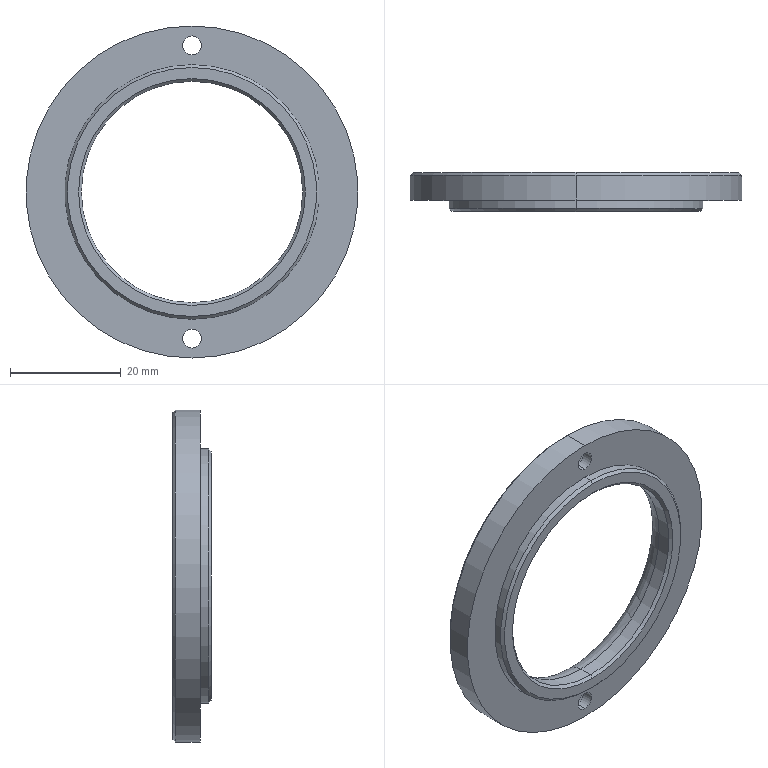Part | SolidWorks | features Chamfer 1, Extrusion 1, Fillet 1, HoleWzd 1, ICE 1 | 1 solid | 28 faces | box 60 x 7 x 60 mm | volume 7951 mm3 | cylinder 14 | cone 6 | plane 6 | torus 2 | commonest cylinder face diameters 3.4 x4 6 x4 40 x2 46 x2 60 x2
STEP:
#1=CARTESIAN_POINT('',(0.,0.5,23.5));
#2=VERTEX_POINT('',#1);
#3=CARTESIAN_POINT('',(0.,0.5,29.5));
#4=VERTEX_POINT('',#3);
#5=CARTESIAN_POINT('',(0.,0.5,26.5));
#6=DIRECTION('',(0.,1.,0.));
#7=DIRECTION('',(0.,0.,1.));
#8=AXIS2_PLACEMENT_3D('',#5,#6,#7);
#9=CIRCLE('',#8,3.);
#10=EDGE_CURVE('',#2,#4,#9,.T.);
#11=ORIENTED_EDGE('',*,*,#10,.F.);
#12=CARTESIAN_POINT('',(0.,3.469,23.5));
#13=VERTEX_POINT('',#12);
#14=CARTESIAN_POINT('',(0.,3.5,23.5));
#15=DIRECTION('',(0.,1.,0.));
#16=VECTOR('',#15,1000.);
#17=LINE('',#14,#16);
#18=EDGE_CURVE('',#2,#13,#17,.T.);
#19=ORIENTED_EDGE('',*,*,#18,.T.);
#20=CARTESIAN_POINT('',(-1.577,3.5,23.948));
#21=VERTEX_POINT('',#20);
#22=CARTESIAN_POINT('',(0.,3.469,23.5));
#23=CARTESIAN_POINT('',(-0.1379,3.469,23.5));
#24=CARTESIAN_POINT('',(-0.2777,3.47,23.51));
#25=CARTESIAN_POINT('',(-0.5518,3.475,23.548));
#26=CARTESIAN_POINT('',(-0.6865,3.479,23.576));
#27=CARTESIAN_POINT('',(-1.083,3.491,23.689));
#28=CARTESIAN_POINT('',(-1.341,3.5,23.802));
#29=CARTESIAN_POINT('',(-1.577,3.5,23.948));
#30=B_SPLINE_CURVE_WITH_KNOTS('',3,(#22,#23,#24,#25,#26,#27,#28,#29),.UNSPECIFIED.,.F.,.F.,(4,2,2,4),(0.00175,0.002163,0.002575,0.0034),.UNSPECIFIED.);
#31=EDGE_CURVE('',#13,#21,#30,.T.);
#32=ORIENTED_EDGE('',*,*,#31,.T.);
#33=CARTESIAN_POINT('',(0.,3.5,29.5));
#34=VERTEX_POINT('',#33);
#35=CARTESIAN_POINT('',(0.,3.5,26.5));
#36=DIRECTION('',(0.,1.,0.));
#37=DIRECTION('',(0.,0.,1.));
#38=AXIS2_PLACEMENT_3D('',#35,#36,#37);
#39=CIRCLE('',#38,3.);
#40=EDGE_CURVE('',#21,#34,#39,.T.);
#41=ORIENTED_EDGE('',*,*,#40,.T.);
#42=CARTESIAN_POINT('',(0.,3.5,29.5));
#43=DIRECTION('',(0.,1.,0.));
#44=VECTOR('',#43,1000.);
#45=LINE('',#42,#44);
#46=EDGE_CURVE('',#4,#34,#45,.T.);
#47=ORIENTED_EDGE('',*,*,#46,.F.);
#48=EDGE_LOOP('',(#11,#19,#32,#41,#47));
#49=FACE_OUTER_BOUND('',#48,.T.);
#50=CARTESIAN_POINT('',(0.,3.5,26.5));
#51=DIRECTION('',(0.,1.,0.));
#52=DIRECTION('',(0.,0.,1.));
#53=AXIS2_PLACEMENT_3D('',#50,#51,#52);
#54=CYLINDRICAL_SURFACE('',#53,3.);
#55=ADVANCED_FACE('',(#49),#54,.F.);
#56=CARTESIAN_POINT('',(0.,-1.5,28.2));
#57=VERTEX_POINT('',#56);
#58=CARTESIAN_POINT('',(0.,-1.5,24.8));
#59=VERTEX_POINT('',#58);
#60=CARTESIAN_POINT('',(0.,-1.5,26.5));
#61=DIRECTION('',(0.,-1.,0.));
#62=DIRECTION('',(0.,0.,-1.));
#63=AXIS2_PLACEMENT_3D('',#60,#61,#62);
#64=CIRCLE('',#63,1.7);
#65=EDGE_CURVE('',#57,#59,#64,.T.);
#66=ORIENTED_EDGE('',*,*,#65,.T.);
#67=CARTESIAN_POINT('',(0.,0.5,24.8));
#68=VERTEX_POINT('',#67);
#69=CARTESIAN_POINT('',(0.,3.5,24.8));
#70=DIRECTION('',(0.,1.,0.));
#71=VECTOR('',#70,1000.);
#72=LINE('',#69,#71);
#73=EDGE_CURVE('',#59,#68,#72,.T.);
#74=ORIENTED_EDGE('',*,*,#73,.T.);
#75=CARTESIAN_POINT('',(0.,0.5,28.2));
#76=VERTEX_POINT('',#75);
#77=CARTESIAN_POINT('',(0.,0.5,26.5));
#78=DIRECTION('',(0.,1.,0.));
#79=DIRECTION('',(0.,0.,1.));
#80=AXIS2_PLACEMENT_3D('',#77,#78,#79);
#81=CIRCLE('',#80,1.7);
#82=EDGE_CURVE('',#68,#76,#81,.T.);
#83=ORIENTED_EDGE('',*,*,#82,.T.);
#84=CARTESIAN_POINT('',(0.,3.5,28.2));
#85=DIRECTION('',(0.,1.,0.));
#86=VECTOR('',#85,1000.);
#87=LINE('',#84,#86);
#88=EDGE_CURVE('',#57,#76,#87,.T.);
#89=ORIENTED_EDGE('',*,*,#88,.F.);
#90=EDGE_LOOP('',(#66,#74,#83,#89));
#91=FACE_OUTER_BOUND('',#90,.T.);
#92=CARTESIAN_POINT('',(0.,3.5,26.5));
#93=DIRECTION('',(0.,1.,0.));
#94=DIRECTION('',(0.,0.,1.));
#95=AXIS2_PLACEMENT_3D('',#92,#93,#94);
#96=CYLINDRICAL_SURFACE('',#95,1.7);
#97=ADVANCED_FACE('',(#91),#96,.F.);
#98=CARTESIAN_POINT('',(0.,0.5,-29.5));
#99=VERTEX_POINT('',#98);
#100=CARTESIAN_POINT('',(0.,0.5,-23.5));
#101=VERTEX_POINT('',#100);
#102=CARTESIAN_POINT('',(0.,0.5,-26.5));
#103=DIRECTION('',(0.,1.,0.));
#104=DIRECTION('',(0.,0.,1.));
#105=AXIS2_PLACEMENT_3D('',#102,#103,#104);
#106=CIRCLE('',#105,3.);
#107=EDGE_CURVE('',#99,#101,#106,.T.);
#108=ORIENTED_EDGE('',*,*,#107,.F.);
#109=CARTESIAN_POINT('',(0.,3.5,-29.5));
#110=VERTEX_POINT('',#109);
#111=CARTESIAN_POINT('',(0.,3.5,-29.5));
#112=DIRECTION('',(0.,1.,0.));
#113=VECTOR('',#112,1000.);
#114=LINE('',#111,#113);
#115=EDGE_CURVE('',#99,#110,#114,.T.);
#116=ORIENTED_EDGE('',*,*,#115,.T.);
#117=CARTESIAN_POINT('',(-1.577,3.5,-23.948));
#118=VERTEX_POINT('',#117);
#119=CARTESIAN_POINT('',(0.,3.5,-26.5));
#120=DIRECTION('',(0.,1.,0.));
#121=DIRECTION('',(0.,0.,1.));
#122=AXIS2_PLACEMENT_3D('',#119,#120,#121);
#123=CIRCLE('',#122,3.);
#124=EDGE_CURVE('',#110,#118,#123,.T.);
#125=ORIENTED_EDGE('',*,*,#124,.T.);
#126=CARTESIAN_POINT('',(0.,3.469,-23.5));
#127=VERTEX_POINT('',#126);
#128=CARTESIAN_POINT('',(-1.577,3.5,-23.948));
#129=CARTESIAN_POINT('',(-1.34,3.5,-23.802));
#130=CARTESIAN_POINT('',(-1.088,3.491,-23.69));
#131=CARTESIAN_POINT('',(-0.5525,3.475,-23.538));
#132=CARTESIAN_POINT('',(-0.2767,3.469,-23.5));
#133=CARTESIAN_POINT('',(0.,3.469,-23.5));
#134=B_SPLINE_CURVE_WITH_KNOTS('',3,(#128,#129,#130,#131,#132,#133),.UNSPECIFIED.,.F.,.F.,(4,2,4),(0.00009543,0.0009229,0.00175),.UNSPECIFIED.);
#135=EDGE_CURVE('',#118,#127,#134,.T.);
#136=ORIENTED_EDGE('',*,*,#135,.T.);
#137=CARTESIAN_POINT('',(0.,3.5,-23.5));
#138=DIRECTION('',(0.,1.,0.));
#139=VECTOR('',#138,1000.);
#140=LINE('',#137,#139);
#141=EDGE_CURVE('',#101,#127,#140,.T.);
#142=ORIENTED_EDGE('',*,*,#141,.F.);
#143=EDGE_LOOP('',(#108,#116,#125,#136,#142));
#144=FACE_OUTER_BOUND('',#143,.T.);
#145=CARTESIAN_POINT('',(0.,3.5,-26.5));
#146=DIRECTION('',(0.,1.,0.));
#147=DIRECTION('',(0.,0.,1.));
#148=AXIS2_PLACEMENT_3D('',#145,#146,#147);
#149=CYLINDRICAL_SURFACE('',#148,3.);
#150=ADVANCED_FACE('',(#144),#149,.F.);
#151=CARTESIAN_POINT('',(0.,-1.5,-24.8));
#152=VERTEX_POINT('',#151);
#153=CARTESIAN_POINT('',(0.,-1.5,-28.2));
#154=VERTEX_POINT('',#153);
#155=CARTESIAN_POINT('',(0.,-1.5,-26.5));
#156=DIRECTION('',(0.,-1.,0.));
#157=DIRECTION('',(0.,0.,-1.));
#158=AXIS2_PLACEMENT_3D('',#155,#156,#157);
#159=CIRCLE('',#158,1.7);
#160=EDGE_CURVE('',#152,#154,#159,.T.);
#161=ORIENTED_EDGE('',*,*,#160,.T.);
#162=CARTESIAN_POINT('',(0.,0.5,-28.2));
#163=VERTEX_POINT('',#162);
#164=CARTESIAN_POINT('',(0.,3.5,-28.2));
#165=DIRECTION('',(0.,1.,0.));
#166=VECTOR('',#165,1000.);
#167=LINE('',#164,#166);
#168=EDGE_CURVE('',#154,#163,#167,.T.);
#169=ORIENTED_EDGE('',*,*,#168,.T.);
#170=CARTESIAN_POINT('',(0.,0.5,-24.8));
#171=VERTEX_POINT('',#170);
#172=CARTESIAN_POINT('',(0.,0.5,-26.5));
#173=DIRECTION('',(0.,1.,0.));
#174=DIRECTION('',(0.,0.,1.));
#175=AXIS2_PLACEMENT_3D('',#172,#173,#174);
#176=CIRCLE('',#175,1.7);
#177=EDGE_CURVE('',#163,#171,#176,.T.);
#178=ORIENTED_EDGE('',*,*,#177,.T.);
#179=CARTESIAN_POINT('',(0.,3.5,-24.8));
#180=DIRECTION('',(0.,1.,0.));
#181=VECTOR('',#180,1000.);
#182=LINE('',#179,#181);
#183=EDGE_CURVE('',#152,#171,#182,.T.);
#184=ORIENTED_EDGE('',*,*,#183,.F.);
#185=EDGE_LOOP('',(#161,#169,#178,#184));
#186=FACE_OUTER_BOUND('',#185,.T.);
#187=CARTESIAN_POINT('',(0.,3.5,-26.5));
#188=DIRECTION('',(0.,1.,0.));
#189=DIRECTION('',(0.,0.,1.));
#190=AXIS2_PLACEMENT_3D('',#187,#188,#189);
#191=CYLINDRICAL_SURFACE('',#190,1.7);
#192=ADVANCED_FACE('',(#186),#191,.F.);
#193=CARTESIAN_POINT('',(0.,-3.5,-22.5));
#194=VERTEX_POINT('',#193);
#195=CARTESIAN_POINT('',(0.,-3.5,22.5));
#196=VERTEX_POINT('',#195);
#197=CARTESIAN_POINT('',(0.,-3.5,0.));
#198=DIRECTION('',(0.,-1.,0.));
#199=DIRECTION('',(0.,0.,1.));
#200=AXIS2_PLACEMENT_3D('',#197,#198,#199);
#201=CIRCLE('',#200,22.5);
#202=EDGE_CURVE('',#194,#196,#201,.T.);
#203=ORIENTED_EDGE('',*,*,#202,.F.);
#204=CARTESIAN_POINT('',(0.,-3.,-23.));
#205=VERTEX_POINT('',#204);
#206=CARTESIAN_POINT('',(0.,-3.5,-22.5));
#207=DIRECTION('',(0.,0.7071,-0.7071));
#208=VECTOR('',#207,1000.);
#209=LINE('',#206,#208);
#210=EDGE_CURVE('',#194,#205,#209,.T.);
#211=ORIENTED_EDGE('',*,*,#210,.T.);
#212=CARTESIAN_POINT('',(0.,-3.,23.));
#213=VERTEX_POINT('',#212);
#214=CARTESIAN_POINT('',(0.,-3.,0.));
#215=DIRECTION('',(0.,1.,0.));
#216=DIRECTION('',(0.,0.,1.));
#217=AXIS2_PLACEMENT_3D('',#214,#215,#216);
#218=CIRCLE('',#217,23.);
#219=EDGE_CURVE('',#213,#205,#218,.T.);
#220=ORIENTED_EDGE('',*,*,#219,.F.);
#221=CARTESIAN_POINT('',(0.,-3.5,22.5));
#222=DIRECTION('',(0.,0.7071,0.7071));
#223=VECTOR('',#222,1000.);
#224=LINE('',#221,#223);
#225=EDGE_CURVE('',#196,#213,#224,.T.);
#226=ORIENTED_EDGE('',*,*,#225,.F.);
#227=EDGE_LOOP('',(#203,#211,#220,#226));
#228=FACE_OUTER_BOUND('',#227,.T.);
#229=CARTESIAN_POINT('',(0.,-3.5,0.));
#230=DIRECTION('',(0.,1.,0.));
#231=DIRECTION('',(0.,0.,1.));
#232=AXIS2_PLACEMENT_3D('',#229,#230,#231);
#233=CONICAL_SURFACE('',#232,22.5,0.7854);
#234=ADVANCED_FACE('',(#228),#233,.T.);
#235=CARTESIAN_POINT('',(0.,-3.,20.));
#236=VERTEX_POINT('',#235);
#237=CARTESIAN_POINT('',(0.,-3.,-20.));
#238=VERTEX_POINT('',#237);
#239=CARTESIAN_POINT('',(0.,-3.,0.));
#240=DIRECTION('',(0.,-1.,0.));
#241=DIRECTION('',(0.,0.,1.));
#242=AXIS2_PLACEMENT_3D('',#239,#240,#241);
#243=CIRCLE('',#242,20.);
#244=EDGE_CURVE('',#236,#238,#243,.T.);
#245=ORIENTED_EDGE('',*,*,#244,.F.);
#246=CARTESIAN_POINT('',(0.,-3.5,20.5));
#247=VERTEX_POINT('',#246);
#248=CARTESIAN_POINT('',(0.,-3.5,20.5));
#249=DIRECTION('',(0.,-0.7071,0.7071));
#250=VECTOR('',#249,1000.);
#251=LINE('',#248,#250);
#252=EDGE_CURVE('',#236,#247,#251,.T.);
#253=ORIENTED_EDGE('',*,*,#252,.T.);
#254=CARTESIAN_POINT('',(0.,-3.5,-20.5));
#255=VERTEX_POINT('',#254);
#256=CARTESIAN_POINT('',(0.,-3.5,0.));
#257=DIRECTION('',(0.,1.,0.));
#258=DIRECTION('',(0.,0.,1.));
#259=AXIS2_PLACEMENT_3D('',#256,#257,#258);
#260=CIRCLE('',#259,20.5);
#261=EDGE_CURVE('',#255,#247,#260,.T.);
#262=ORIENTED_EDGE('',*,*,#261,.F.);
#263=CARTESIAN_POINT('',(0.,-3.5,-20.5));
#264=DIRECTION('',(0.,-0.7071,-0.7071));
#265=VECTOR('',#264,1000.);
#266=LINE('',#263,#265);
#267=EDGE_CURVE('',#238,#255,#266,.T.);
#268=ORIENTED_EDGE('',*,*,#267,.F.);
#269=EDGE_LOOP('',(#245,#253,#262,#268));
#270=FACE_OUTER_BOUND('',#269,.T.);
#271=CARTESIAN_POINT('',(0.,-3.5,0.));
#272=DIRECTION('',(0.,-1.,0.));
#273=DIRECTION('',(0.,0.,-1.));
#274=AXIS2_PLACEMENT_3D('',#271,#272,#273);
#275=CONICAL_SURFACE('',#274,20.5,0.7854);
#276=ADVANCED_FACE('',(#270),#275,.F.);
#277=CARTESIAN_POINT('',(0.,3.5,0.));
#278=DIRECTION('',(0.,1.,0.));
#279=DIRECTION('',(0.,0.,1.));
#280=AXIS2_PLACEMENT_3D('',#277,#278,#279);
#281=CIRCLE('',#280,29.5);
#282=EDGE_CURVE('',#34,#110,#281,.T.);
#283=ORIENTED_EDGE('',*,*,#282,.F.);
#284=CARTESIAN_POINT('',(0.,3.,30.));
#285=VERTEX_POINT('',#284);
#286=CARTESIAN_POINT('',(0.,3.5,29.5));
#287=DIRECTION('',(0.,-0.7071,0.7071));
#288=VECTOR('',#287,1000.);
#289=LINE('',#286,#288);
#290=EDGE_CURVE('',#34,#285,#289,.T.);
#291=ORIENTED_EDGE('',*,*,#290,.T.);
#292=CARTESIAN_POINT('',(0.,3.,-30.));
#293=VERTEX_POINT('',#292);
#294=CARTESIAN_POINT('',(0.,3.,0.));
#295=DIRECTION('',(0.,-1.,0.));
#296=DIRECTION('',(0.,0.,1.));
#297=AXIS2_PLACEMENT_3D('',#294,#295,#296);
#298=CIRCLE('',#297,30.);
#299=EDGE_CURVE('',#293,#285,#298,.T.);
#300=ORIENTED_EDGE('',*,*,#299,.F.);
#301=CARTESIAN_POINT('',(0.,3.5,-29.5));
#302=DIRECTION('',(0.,-0.7071,-0.7071));
#303=VECTOR('',#302,1000.);
#304=LINE('',#301,#303);
#305=EDGE_CURVE('',#110,#293,#304,.T.);
#306=ORIENTED_EDGE('',*,*,#305,.F.);
#307=EDGE_LOOP('',(#283,#291,#300,#306));
#308=FACE_OUTER_BOUND('',#307,.T.);
#309=CARTESIAN_POINT('',(0.,3.5,0.));
#310=DIRECTION('',(0.,-1.,0.));
#311=DIRECTION('',(0.,0.,-1.));
#312=AXIS2_PLACEMENT_3D('',#309,#310,#311);
#313=CONICAL_SURFACE('',#312,29.5,0.7854);
#314=ADVANCED_FACE('',(#308),#313,.T.);
#315=CARTESIAN_POINT('',(1.577,3.5,-23.948));
#316=VERTEX_POINT('',#315);
#317=CARTESIAN_POINT('',(0.,3.469,-23.5));
#318=CARTESIAN_POINT('',(0.1379,3.469,-23.5));
#319=CARTESIAN_POINT('',(0.2777,3.47,-23.51));
#320=CARTESIAN_POINT('',(0.5518,3.475,-23.548));
#321=CARTESIAN_POINT('',(0.6865,3.479,-23.576));
#322=CARTESIAN_POINT('',(1.083,3.491,-23.689));
#323=CARTESIAN_POINT('',(1.341,3.5,-23.802));
#324=CARTESIAN_POINT('',(1.577,3.5,-23.948));
#325=B_SPLINE_CURVE_WITH_KNOTS('',3,(#317,#318,#319,#320,#321,#322,#323,#324),.UNSPECIFIED.,.F.,.F.,(4,2,2,4),(0.00175,0.002163,0.002575,0.0034),.UNSPECIFIED.);
#326=EDGE_CURVE('',#127,#316,#325,.T.);
#327=ORIENTED_EDGE('',*,*,#326,.F.);
#328=CARTESIAN_POINT('',(0.,-0.5,-20.));
#329=VERTEX_POINT('',#328);
#330=CARTESIAN_POINT('',(0.,-0.5,-24.));
#331=DIRECTION('',(1.,0.,0.));
#332=DIRECTION('',(0.,0.,-1.));
#333=AXIS2_PLACEMENT_3D('',#330,#331,#332);
#334=CIRCLE('',#333,4.);
#335=EDGE_CURVE('',#127,#329,#334,.T.);
#336=ORIENTED_EDGE('',*,*,#335,.T.);
#337=CARTESIAN_POINT('',(0.,-0.5,20.));
#338=VERTEX_POINT('',#337);
#339=CARTESIAN_POINT('',(0.,-0.5,0.));
#340=DIRECTION('',(0.,1.,0.));
#341=DIRECTION('',(0.,0.,1.));
#342=AXIS2_PLACEMENT_3D('',#339,#340,#341);
#343=CIRCLE('',#342,20.);
#344=EDGE_CURVE('',#338,#329,#343,.T.);
#345=ORIENTED_EDGE('',*,*,#344,.F.);
#346=CARTESIAN_POINT('',(0.,-0.5,24.));
#347=DIRECTION('',(-1.,0.,0.));
#348=DIRECTION('',(0.,0.,1.));
#349=AXIS2_PLACEMENT_3D('',#346,#347,#348);
#350=CIRCLE('',#349,4.);
#351=EDGE_CURVE('',#13,#338,#350,.T.);
#352=ORIENTED_EDGE('',*,*,#351,.F.);
#353=CARTESIAN_POINT('',(1.577,3.5,23.948));
#354=VERTEX_POINT('',#353);
#355=CARTESIAN_POINT('',(1.577,3.5,23.948));
#356=CARTESIAN_POINT('',(1.34,3.5,23.802));
#357=CARTESIAN_POINT('',(1.088,3.491,23.69));
#358=CARTESIAN_POINT('',(0.5525,3.475,23.538));
#359=CARTESIAN_POINT('',(0.2767,3.469,23.5));
#360=CARTESIAN_POINT('',(0.,3.469,23.5));
#361=B_SPLINE_CURVE_WITH_KNOTS('',3,(#355,#356,#357,#358,#359,#360),.UNSPECIFIED.,.F.,.F.,(4,2,4),(0.00009543,0.0009229,0.00175),.UNSPECIFIED.);
#362=EDGE_CURVE('',#354,#13,#361,.T.);
#363=ORIENTED_EDGE('',*,*,#362,.F.);
#364=CARTESIAN_POINT('',(0.,3.5,0.));
#365=DIRECTION('',(0.,-1.,0.));
#366=DIRECTION('',(0.,0.,1.));
#367=AXIS2_PLACEMENT_3D('',#364,#365,#366);
#368=CIRCLE('',#367,24.);
#369=EDGE_CURVE('',#316,#354,#368,.T.);
#370=ORIENTED_EDGE('',*,*,#369,.F.);
#371=EDGE_LOOP('',(#327,#336,#345,#352,#363,#370));
#372=FACE_OUTER_BOUND('',#371,.T.);
#373=CARTESIAN_POINT('',(0.,-0.5,0.));
#374=DIRECTION('',(0.,1.,0.));
#375=DIRECTION('',(0.,0.,1.));
#376=AXIS2_PLACEMENT_3D('',#373,#374,#375);
#377=TOROIDAL_SURFACE('',#376,24.,4.);
#378=ADVANCED_FACE('',(#372),#377,.T.);
#379=CARTESIAN_POINT('',(0.,-1.5,-23.));
#380=VERTEX_POINT('',#379);
#381=CARTESIAN_POINT('',(0.,-1.5,23.));
#382=VERTEX_POINT('',#381);
#383=CARTESIAN_POINT('',(0.,-1.5,0.));
#384=DIRECTION('',(0.,-1.,0.));
#385=DIRECTION('',(0.,0.,-1.));
#386=AXIS2_PLACEMENT_3D('',#383,#384,#385);
#387=CIRCLE('',#386,23.);
#388=EDGE_CURVE('',#380,#382,#387,.T.);
#389=ORIENTED_EDGE('',*,*,#388,.T.);
#390=CARTESIAN_POINT('',(0.,-1.5,23.));
#391=DIRECTION('',(0.,-1.,0.));
#392=VECTOR('',#391,1000.);
#393=LINE('',#390,#392);
#394=EDGE_CURVE('',#382,#213,#393,.T.);
#395=ORIENTED_EDGE('',*,*,#394,.T.);
#396=ORIENTED_EDGE('',*,*,#219,.T.);
#397=CARTESIAN_POINT('',(0.,-1.5,-23.));
#398=DIRECTION('',(0.,-1.,0.));
#399=VECTOR('',#398,1000.);
#400=LINE('',#397,#399);
#401=EDGE_CURVE('',#380,#205,#400,.T.);
#402=ORIENTED_EDGE('',*,*,#401,.F.);
#403=EDGE_LOOP('',(#389,#395,#396,#402));
#404=FACE_OUTER_BOUND('',#403,.T.);
#405=CARTESIAN_POINT('',(0.,-1.5,0.));
#406=DIRECTION('',(0.,-1.,0.));
#407=DIRECTION('',(0.,0.,-1.));
#408=AXIS2_PLACEMENT_3D('',#405,#406,#407);
#409=CYLINDRICAL_SURFACE('',#408,23.);
#410=ADVANCED_FACE('',(#404),#409,.T.);
#411=CARTESIAN_POINT('',(0.,-0.5,0.));
#412=DIRECTION('',(0.,1.,0.));
#413=DIRECTION('',(0.,0.,1.));
#414=AXIS2_PLACEMENT_3D('',#411,#412,#413);
#415=CIRCLE('',#414,20.);
#416=EDGE_CURVE('',#329,#338,#415,.T.);
#417=ORIENTED_EDGE('',*,*,#416,.T.);
#418=CARTESIAN_POINT('',(0.,3.5,20.));
#419=DIRECTION('',(0.,-1.,0.));
#420=VECTOR('',#419,1000.);
#421=LINE('',#418,#420);
#422=EDGE_CURVE('',#338,#236,#421,.T.);
#423=ORIENTED_EDGE('',*,*,#422,.T.);
#424=ORIENTED_EDGE('',*,*,#244,.T.);
#425=CARTESIAN_POINT('',(0.,3.5,-20.));
#426=DIRECTION('',(0.,-1.,0.));
#427=VECTOR('',#426,1000.);
#428=LINE('',#425,#427);
#429=EDGE_CURVE('',#329,#238,#428,.T.);
#430=ORIENTED_EDGE('',*,*,#429,.F.);
#431=EDGE_LOOP('',(#417,#423,#424,#430));
#432=FACE_OUTER_BOUND('',#431,.T.);
#433=CARTESIAN_POINT('',(0.,3.5,0.));
#434=DIRECTION('',(0.,-1.,0.));
#435=DIRECTION('',(0.,0.,-1.));
#436=AXIS2_PLACEMENT_3D('',#433,#434,#435);
#437=CYLINDRICAL_SURFACE('',#436,20.);
#438=ADVANCED_FACE('',(#432),#437,.F.);
#439=ORIENTED_EDGE('',*,*,#299,.T.);
#440=CARTESIAN_POINT('',(0.,-1.5,30.));
#441=VERTEX_POINT('',#440);
#442=CARTESIAN_POINT('',(0.,3.5,30.));
#443=DIRECTION('',(0.,-1.,0.));
#444=VECTOR('',#443,1000.);
#445=LINE('',#442,#444);
#446=EDGE_CURVE('',#285,#441,#445,.T.);
#447=ORIENTED_EDGE('',*,*,#446,.T.);
#448=CARTESIAN_POINT('',(0.,-1.5,-30.));
#449=VERTEX_POINT('',#448);
#450=CARTESIAN_POINT('',(0.,-1.5,0.));
#451=DIRECTION('',(0.,-1.,0.));
#452=DIRECTION('',(0.,0.,-1.));
#453=AXIS2_PLACEMENT_3D('',#450,#451,#452);
#454=CIRCLE('',#453,30.);
#455=EDGE_CURVE('',#449,#441,#454,.T.);
#456=ORIENTED_EDGE('',*,*,#455,.F.);
#457=CARTESIAN_POINT('',(0.,3.5,-30.));
#458=DIRECTION('',(0.,-1.,0.));
#459=VECTOR('',#458,1000.);
#460=LINE('',#457,#459);
#461=EDGE_CURVE('',#293,#449,#460,.T.);
#462=ORIENTED_EDGE('',*,*,#461,.F.);
#463=EDGE_LOOP('',(#439,#447,#456,#462));
#464=FACE_OUTER_BOUND('',#463,.T.);
#465=CARTESIAN_POINT('',(0.,3.5,0.));
#466=DIRECTION('',(0.,-1.,0.));
#467=DIRECTION('',(0.,0.,-1.));
#468=AXIS2_PLACEMENT_3D('',#465,#466,#467);
#469=CYLINDRICAL_SURFACE('',#468,30.);
#470=ADVANCED_FACE('',(#464),#469,.T.);
#471=CARTESIAN_POINT('',(0.,3.5,26.5));
#472=DIRECTION('',(0.,1.,0.));
#473=DIRECTION('',(0.,0.,1.));
#474=AXIS2_PLACEMENT_3D('',#471,#472,#473);
#475=CIRCLE('',#474,3.);
#476=EDGE_CURVE('',#34,#354,#475,.T.);
#477=ORIENTED_EDGE('',*,*,#476,.F.);
#478=ORIENTED_EDGE('',*,*,#282,.T.);
#479=CARTESIAN_POINT('',(0.,3.5,-26.5));
#480=DIRECTION('',(0.,1.,0.));
#481=DIRECTION('',(0.,0.,1.));
#482=AXIS2_PLACEMENT_3D('',#479,#480,#481);
#483=CIRCLE('',#482,3.);
#484=EDGE_CURVE('',#316,#110,#483,.T.);
#485=ORIENTED_EDGE('',*,*,#484,.F.);
#486=ORIENTED_EDGE('',*,*,#369,.T.);
#487=EDGE_LOOP('',(#477,#478,#485,#486));
#488=FACE_OUTER_BOUND('',#487,.T.);
#489=CARTESIAN_POINT('',(0.,3.5,0.));
#490=DIRECTION('',(0.,1.,0.));
#491=DIRECTION('',(0.,0.,1.));
#492=AXIS2_PLACEMENT_3D('',#489,#490,#491);
#493=PLANE('',#492);
#494=ADVANCED_FACE('',(#488),#493,.T.);
#495=ORIENTED_EDGE('',*,*,#261,.T.);
#496=CARTESIAN_POINT('',(0.,-3.5,0.));
#497=DIRECTION('',(0.,1.,0.));
#498=DIRECTION('',(0.,0.,1.));
#499=AXIS2_PLACEMENT_3D('',#496,#497,#498);
#500=CIRCLE('',#499,20.5);
#501=EDGE_CURVE('',#247,#255,#500,.T.);
#502=ORIENTED_EDGE('',*,*,#501,.T.);
#503=EDGE_LOOP('',(#495,#502));
#504=FACE_BOUND('',#503,.T.);
#505=CARTESIAN_POINT('',(0.,-3.5,0.));
#506=DIRECTION('',(0.,-1.,0.));
#507=DIRECTION('',(0.,0.,1.));
#508=AXIS2_PLACEMENT_3D('',#505,#506,#507);
#509=CIRCLE('',#508,22.5);
#510=EDGE_CURVE('',#196,#194,#509,.T.);
#511=ORIENTED_EDGE('',*,*,#510,.T.);
#512=ORIENTED_EDGE('',*,*,#202,.T.);
#513=EDGE_LOOP('',(#511,#512));
#514=FACE_OUTER_BOUND('',#513,.T.);
#515=CARTESIAN_POINT('',(0.,-3.5,0.));
#516=DIRECTION('',(0.,1.,0.));
#517=DIRECTION('',(0.,0.,1.));
#518=AXIS2_PLACEMENT_3D('',#515,#516,#517);
#519=PLANE('',#518);
#520=ADVANCED_FACE('',(#504,#514),#519,.F.);
#521=ORIENTED_EDGE('',*,*,#446,.F.);
#522=CARTESIAN_POINT('',(0.,3.,0.));
#523=DIRECTION('',(0.,-1.,0.));
#524=DIRECTION('',(0.,0.,1.));
#525=AXIS2_PLACEMENT_3D('',#522,#523,#524);
#526=CIRCLE('',#525,30.);
#527=EDGE_CURVE('',#285,#293,#526,.T.);
#528=ORIENTED_EDGE('',*,*,#527,.T.);
#529=ORIENTED_EDGE('',*,*,#461,.T.);
#530=CARTESIAN_POINT('',(0.,-1.5,0.));
#531=DIRECTION('',(0.,-1.,0.));
#532=DIRECTION('',(0.,0.,-1.));
#533=AXIS2_PLACEMENT_3D('',#530,#531,#532);
#534=CIRCLE('',#533,30.);
#535=EDGE_CURVE('',#441,#449,#534,.T.);
#536=ORIENTED_EDGE('',*,*,#535,.F.);
#537=EDGE_LOOP('',(#521,#528,#529,#536));
#538=FACE_OUTER_BOUND('',#537,.T.);
#539=CARTESIAN_POINT('',(0.,3.5,0.));
#540=DIRECTION('',(0.,-1.,0.));
#541=DIRECTION('',(0.,0.,-1.));
#542=AXIS2_PLACEMENT_3D('',#539,#540,#541);
#543=CYLINDRICAL_SURFACE('',#542,30.);
#544=ADVANCED_FACE('',(#538),#543,.T.);
#545=ORIENTED_EDGE('',*,*,#40,.F.);
#546=CARTESIAN_POINT('',(0.,3.5,0.));
#547=DIRECTION('',(0.,-1.,0.));
#548=DIRECTION('',(0.,0.,1.));
#549=AXIS2_PLACEMENT_3D('',#546,#547,#548);
#550=CIRCLE('',#549,24.);
#551=EDGE_CURVE('',#21,#118,#550,.T.);
#552=ORIENTED_EDGE('',*,*,#551,.T.);
#553=ORIENTED_EDGE('',*,*,#124,.F.);
#554=CARTESIAN_POINT('',(0.,3.5,0.));
#555=DIRECTION('',(0.,1.,0.));
#556=DIRECTION('',(0.,0.,1.));
#557=AXIS2_PLACEMENT_3D('',#554,#555,#556);
#558=CIRCLE('',#557,29.5);
#559=EDGE_CURVE('',#110,#34,#558,.T.);
#560=ORIENTED_EDGE('',*,*,#559,.T.);
#561=EDGE_LOOP('',(#545,#552,#553,#560));
#562=FACE_OUTER_BOUND('',#561,.T.);
#563=CARTESIAN_POINT('',(0.,3.5,0.));
#564=DIRECTION('',(0.,1.,0.));
#565=DIRECTION('',(0.,0.,1.));
#566=AXIS2_PLACEMENT_3D('',#563,#564,#565);
#567=PLANE('',#566);
#568=ADVANCED_FACE('',(#562),#567,.T.);
#569=ORIENTED_EDGE('',*,*,#422,.F.);
#570=ORIENTED_EDGE('',*,*,#344,.T.);
#571=ORIENTED_EDGE('',*,*,#429,.T.);
#572=CARTESIAN_POINT('',(0.,-3.,0.));
#573=DIRECTION('',(0.,-1.,0.));
#574=DIRECTION('',(0.,0.,1.));
#575=AXIS2_PLACEMENT_3D('',#572,#573,#574);
#576=CIRCLE('',#575,20.);
#577=EDGE_CURVE('',#238,#236,#576,.T.);
#578=ORIENTED_EDGE('',*,*,#577,.T.);
#579=EDGE_LOOP('',(#569,#570,#571,#578));
#580=FACE_OUTER_BOUND('',#579,.T.);
#581=CARTESIAN_POINT('',(0.,3.5,0.));
#582=DIRECTION('',(0.,-1.,0.));
#583=DIRECTION('',(0.,0.,-1.));
#584=AXIS2_PLACEMENT_3D('',#581,#582,#583);
#585=CYLINDRICAL_SURFACE('',#584,20.);
#586=ADVANCED_FACE('',(#580),#585,.F.);
#587=ORIENTED_EDGE('',*,*,#65,.F.);
#588=CARTESIAN_POINT('',(0.,-1.5,26.5));
#589=DIRECTION('',(0.,-1.,0.));
#590=DIRECTION('',(0.,0.,-1.));
#591=AXIS2_PLACEMENT_3D('',#588,#589,#590);
#592=CIRCLE('',#591,1.7);
#593=EDGE_CURVE('',#59,#57,#592,.T.);
#594=ORIENTED_EDGE('',*,*,#593,.F.);
#595=EDGE_LOOP('',(#587,#594));
#596=FACE_BOUND('',#595,.T.);
#597=ORIENTED_EDGE('',*,*,#160,.F.);
#598=CARTESIAN_POINT('',(0.,-1.5,-26.5));
#599=DIRECTION('',(0.,-1.,0.));
#600=DIRECTION('',(0.,0.,-1.));
#601=AXIS2_PLACEMENT_3D('',#598,#599,#600);
#602=CIRCLE('',#601,1.7);
#603=EDGE_CURVE('',#154,#152,#602,.T.);
#604=ORIENTED_EDGE('',*,*,#603,.F.);
#605=EDGE_LOOP('',(#597,#604));
#606=FACE_BOUND('',#605,.T.);
#607=ORIENTED_EDGE('',*,*,#388,.F.);
#608=CARTESIAN_POINT('',(0.,-1.5,0.));
#609=DIRECTION('',(0.,-1.,0.));
#610=DIRECTION('',(0.,0.,-1.));
#611=AXIS2_PLACEMENT_3D('',#608,#609,#610);
#612=CIRCLE('',#611,23.);
#613=EDGE_CURVE('',#382,#380,#612,.T.);
#614=ORIENTED_EDGE('',*,*,#613,.F.);
#615=EDGE_LOOP('',(#607,#614));
#616=FACE_BOUND('',#615,.T.);
#617=ORIENTED_EDGE('',*,*,#455,.T.);
#618=ORIENTED_EDGE('',*,*,#535,.T.);
#619=EDGE_LOOP('',(#617,#618));
#620=FACE_OUTER_BOUND('',#619,.T.);
#621=CARTESIAN_POINT('',(0.,-1.5,0.));
#622=DIRECTION('',(0.,-1.,0.));
#623=DIRECTION('',(0.,0.,-1.));
#624=AXIS2_PLACEMENT_3D('',#621,#622,#623);
#625=PLANE('',#624);
#626=ADVANCED_FACE('',(#596,#606,#616,#620),#625,.T.);
#627=ORIENTED_EDGE('',*,*,#394,.F.);
#628=ORIENTED_EDGE('',*,*,#613,.T.);
#629=ORIENTED_EDGE('',*,*,#401,.T.);
#630=CARTESIAN_POINT('',(0.,-3.,0.));
#631=DIRECTION('',(0.,1.,0.));
#632=DIRECTION('',(0.,0.,1.));
#633=AXIS2_PLACEMENT_3D('',#630,#631,#632);
#634=CIRCLE('',#633,23.);
#635=EDGE_CURVE('',#205,#213,#634,.T.);
#636=ORIENTED_EDGE('',*,*,#635,.T.);
#637=EDGE_LOOP('',(#627,#628,#629,#636));
#638=FACE_OUTER_BOUND('',#637,.T.);
#639=CARTESIAN_POINT('',(0.,-1.5,0.));
#640=DIRECTION('',(0.,-1.,0.));
#641=DIRECTION('',(0.,0.,-1.));
#642=AXIS2_PLACEMENT_3D('',#639,#640,#641);
#643=CYLINDRICAL_SURFACE('',#642,23.);
#644=ADVANCED_FACE('',(#638),#643,.T.);
#645=ORIENTED_EDGE('',*,*,#335,.F.);
#646=ORIENTED_EDGE('',*,*,#135,.F.);
#647=ORIENTED_EDGE('',*,*,#551,.F.);
#648=ORIENTED_EDGE('',*,*,#31,.F.);
#649=ORIENTED_EDGE('',*,*,#351,.T.);
#650=ORIENTED_EDGE('',*,*,#416,.F.);
#651=EDGE_LOOP('',(#645,#646,#647,#648,#649,#650));
#652=FACE_OUTER_BOUND('',#651,.T.);
#653=CARTESIAN_POINT('',(0.,-0.5,0.));
#654=DIRECTION('',(0.,1.,0.));
#655=DIRECTION('',(0.,0.,1.));
#656=AXIS2_PLACEMENT_3D('',#653,#654,#655);
#657=TOROIDAL_SURFACE('',#656,24.,4.);
#658=ADVANCED_FACE('',(#652),#657,.T.);
#659=ORIENTED_EDGE('',*,*,#290,.F.);
#660=ORIENTED_EDGE('',*,*,#559,.F.);
#661=ORIENTED_EDGE('',*,*,#305,.T.);
#662=ORIENTED_EDGE('',*,*,#527,.F.);
#663=EDGE_LOOP('',(#659,#660,#661,#662));
#664=FACE_OUTER_BOUND('',#663,.T.);
#665=CARTESIAN_POINT('',(0.,3.5,0.));
#666=DIRECTION('',(0.,-1.,0.));
#667=DIRECTION('',(0.,0.,-1.));
#668=AXIS2_PLACEMENT_3D('',#665,#666,#667);
#669=CONICAL_SURFACE('',#668,29.5,0.7854);
#670=ADVANCED_FACE('',(#664),#669,.T.);
#671=ORIENTED_EDGE('',*,*,#252,.F.);
#672=ORIENTED_EDGE('',*,*,#577,.F.);
#673=ORIENTED_EDGE('',*,*,#267,.T.);
#674=ORIENTED_EDGE('',*,*,#501,.F.);
#675=EDGE_LOOP('',(#671,#672,#673,#674));
#676=FACE_OUTER_BOUND('',#675,.T.);
#677=CARTESIAN_POINT('',(0.,-3.5,0.));
#678=DIRECTION('',(0.,-1.,0.));
#679=DIRECTION('',(0.,0.,-1.));
#680=AXIS2_PLACEMENT_3D('',#677,#678,#679);
#681=CONICAL_SURFACE('',#680,20.5,0.7854);
#682=ADVANCED_FACE('',(#676),#681,.F.);
#683=ORIENTED_EDGE('',*,*,#210,.F.);
#684=ORIENTED_EDGE('',*,*,#510,.F.);
#685=ORIENTED_EDGE('',*,*,#225,.T.);
#686=ORIENTED_EDGE('',*,*,#635,.F.);
#687=EDGE_LOOP('',(#683,#684,#685,#686));
#688=FACE_OUTER_BOUND('',#687,.T.);
#689=CARTESIAN_POINT('',(0.,-3.5,0.));
#690=DIRECTION('',(0.,1.,0.));
#691=DIRECTION('',(0.,0.,1.));
#692=AXIS2_PLACEMENT_3D('',#689,#690,#691);
#693=CONICAL_SURFACE('',#692,22.5,0.7854);
#694=ADVANCED_FACE('',(#688),#693,.T.);
#695=ORIENTED_EDGE('',*,*,#168,.F.);
#696=ORIENTED_EDGE('',*,*,#603,.T.);
#697=ORIENTED_EDGE('',*,*,#183,.T.);
#698=CARTESIAN_POINT('',(0.,0.5,-26.5));
#699=DIRECTION('',(0.,1.,0.));
#700=DIRECTION('',(0.,0.,1.));
#701=AXIS2_PLACEMENT_3D('',#698,#699,#700);
#702=CIRCLE('',#701,1.7);
#703=EDGE_CURVE('',#171,#163,#702,.T.);
#704=ORIENTED_EDGE('',*,*,#703,.T.);
#705=EDGE_LOOP('',(#695,#696,#697,#704));
#706=FACE_OUTER_BOUND('',#705,.T.);
#707=CARTESIAN_POINT('',(0.,3.5,-26.5));
#708=DIRECTION('',(0.,1.,0.));
#709=DIRECTION('',(0.,0.,1.));
#710=AXIS2_PLACEMENT_3D('',#707,#708,#709);
#711=CYLINDRICAL_SURFACE('',#710,1.7);
#712=ADVANCED_FACE('',(#706),#711,.F.);
#713=ORIENTED_EDGE('',*,*,#703,.F.);
#714=ORIENTED_EDGE('',*,*,#177,.F.);
#715=EDGE_LOOP('',(#713,#714));
#716=FACE_BOUND('',#715,.T.);
#717=CARTESIAN_POINT('',(0.,0.5,-26.5));
#718=DIRECTION('',(0.,1.,0.));
#719=DIRECTION('',(0.,0.,1.));
#720=AXIS2_PLACEMENT_3D('',#717,#718,#719);
#721=CIRCLE('',#720,3.);
#722=EDGE_CURVE('',#101,#99,#721,.T.);
#723=ORIENTED_EDGE('',*,*,#722,.T.);
#724=ORIENTED_EDGE('',*,*,#107,.T.);
#725=EDGE_LOOP('',(#723,#724));
#726=FACE_OUTER_BOUND('',#725,.T.);
#727=CARTESIAN_POINT('',(1.7,0.5,-26.5));
#728=DIRECTION('',(0.,-1.,0.));
#729=DIRECTION('',(0.,0.,-1.));
#730=AXIS2_PLACEMENT_3D('',#727,#728,#729);
#731=PLANE('',#730);
#732=ADVANCED_FACE('',(#716,#726),#731,.F.);
#733=ORIENTED_EDGE('',*,*,#115,.F.);
#734=ORIENTED_EDGE('',*,*,#722,.F.);
#735=ORIENTED_EDGE('',*,*,#141,.T.);
#736=ORIENTED_EDGE('',*,*,#326,.T.);
#737=ORIENTED_EDGE('',*,*,#484,.T.);
#738=EDGE_LOOP('',(#733,#734,#735,#736,#737));
#739=FACE_OUTER_BOUND('',#738,.T.);
#740=CARTESIAN_POINT('',(0.,3.5,-26.5));
#741=DIRECTION('',(0.,1.,0.));
#742=DIRECTION('',(0.,0.,1.));
#743=AXIS2_PLACEMENT_3D('',#740,#741,#742);
#744=CYLINDRICAL_SURFACE('',#743,3.);
#745=ADVANCED_FACE('',(#739),#744,.F.);
#746=ORIENTED_EDGE('',*,*,#73,.F.);
#747=ORIENTED_EDGE('',*,*,#593,.T.);
#748=ORIENTED_EDGE('',*,*,#88,.T.);
#749=CARTESIAN_POINT('',(0.,0.5,26.5));
#750=DIRECTION('',(0.,1.,0.));
#751=DIRECTION('',(0.,0.,1.));
#752=AXIS2_PLACEMENT_3D('',#749,#750,#751);
#753=CIRCLE('',#752,1.7);
#754=EDGE_CURVE('',#76,#68,#753,.T.);
#755=ORIENTED_EDGE('',*,*,#754,.T.);
#756=EDGE_LOOP('',(#746,#747,#748,#755));
#757=FACE_OUTER_BOUND('',#756,.T.);
#758=CARTESIAN_POINT('',(0.,3.5,26.5));
#759=DIRECTION('',(0.,1.,0.));
#760=DIRECTION('',(0.,0.,1.));
#761=AXIS2_PLACEMENT_3D('',#758,#759,#760);
#762=CYLINDRICAL_SURFACE('',#761,1.7);
#763=ADVANCED_FACE('',(#757),#762,.F.);
#764=ORIENTED_EDGE('',*,*,#754,.F.);
#765=ORIENTED_EDGE('',*,*,#82,.F.);
#766=EDGE_LOOP('',(#764,#765));
#767=FACE_BOUND('',#766,.T.);
#768=CARTESIAN_POINT('',(0.,0.5,26.5));
#769=DIRECTION('',(0.,1.,0.));
#770=DIRECTION('',(0.,0.,1.));
#771=AXIS2_PLACEMENT_3D('',#768,#769,#770);
#772=CIRCLE('',#771,3.);
#773=EDGE_CURVE('',#4,#2,#772,.T.);
#774=ORIENTED_EDGE('',*,*,#773,.T.);
#775=ORIENTED_EDGE('',*,*,#10,.T.);
#776=EDGE_LOOP('',(#774,#775));
#777=FACE_OUTER_BOUND('',#776,.T.);
#778=CARTESIAN_POINT('',(1.7,0.5,26.5));
#779=DIRECTION('',(0.,-1.,0.));
#780=DIRECTION('',(0.,0.,-1.));
#781=AXIS2_PLACEMENT_3D('',#778,#779,#780);
#782=PLANE('',#781);
#783=ADVANCED_FACE('',(#767,#777),#782,.F.);
#784=ORIENTED_EDGE('',*,*,#18,.F.);
#785=ORIENTED_EDGE('',*,*,#773,.F.);
#786=ORIENTED_EDGE('',*,*,#46,.T.);
#787=ORIENTED_EDGE('',*,*,#476,.T.);
#788=ORIENTED_EDGE('',*,*,#362,.T.);
#789=EDGE_LOOP('',(#784,#785,#786,#787,#788));
#790=FACE_OUTER_BOUND('',#789,.T.);
#791=CARTESIAN_POINT('',(0.,3.5,26.5));
#792=DIRECTION('',(0.,1.,0.));
#793=DIRECTION('',(0.,0.,1.));
#794=AXIS2_PLACEMENT_3D('',#791,#792,#793);
#795=CYLINDRICAL_SURFACE('',#794,3.);
#796=ADVANCED_FACE('',(#790),#795,.F.);
#797=CLOSED_SHELL('',(#55,#97,#150,#192,#234,#276,#314,#378,#410,#438,#470,#494,#520,#544,#568,#586,#626,#644,#658,#670,#682,#694,#712,#732,#745,#763,#783,#796));
#798=MANIFOLD_SOLID_BREP('',#797);
#799=CARTESIAN_POINT('',(0.,0.,0.));
#800=DIRECTION('',(0.,0.,1.));
#801=DIRECTION('',(1.,0.,0.));
#802=AXIS2_PLACEMENT_3D('',#799,#800,#801);
#803=(LENGTH_UNIT()NAMED_UNIT(*)SI_UNIT(.MILLI.,.METRE.));
#804=UNCERTAINTY_MEASURE_WITH_UNIT(LENGTH_MEASURE(0.00001),#803,'','');
#805=(NAMED_UNIT(*)PLANE_ANGLE_UNIT()SI_UNIT($,.RADIAN.));
#806=(NAMED_UNIT(*)SI_UNIT($,.STERADIAN.)SOLID_ANGLE_UNIT());
#807=(GEOMETRIC_REPRESENTATION_CONTEXT(3)GLOBAL_UNCERTAINTY_ASSIGNED_CONTEXT((#804))GLOBAL_UNIT_ASSIGNED_CONTEXT((#803,#805,#806))REPRESENTATION_CONTEXT('',''));
#808=ADVANCED_BREP_SHAPE_REPRESENTATION('',(#798,#802),#807);